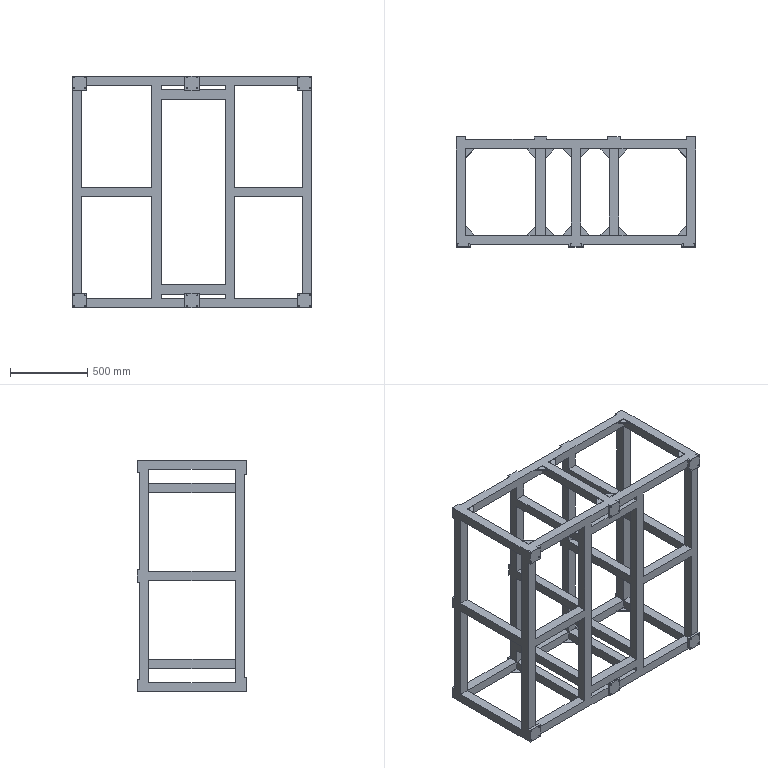Part | STEP file | 09-16 lower frame | 1 solid | 356 faces | box 1550 x 710 x 1500 mm | volume 100220084 mm3 | plane 228 | cylinder 72 | cone 56 | commonest cylinder face diameters 6.8 x72